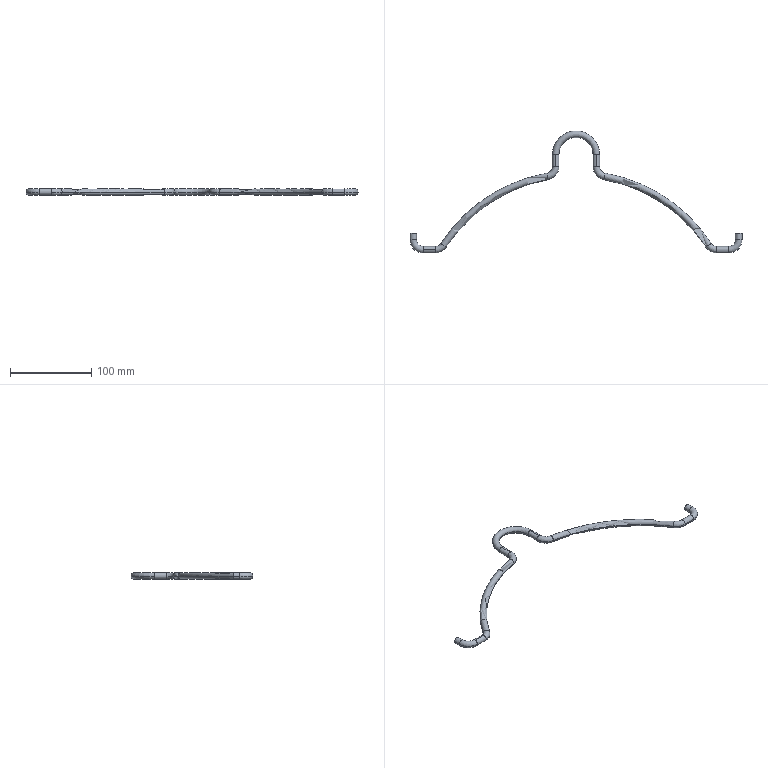Part | STEP file | HXGR200008-05-20-03 | 1 solid | 32 faces | box 408 x 150 x 8 mm | volume 28410 mm3 | torus 18 | cylinder 12 | plane 2 | commonest cylinder face diameters 8 x12
STEP:
#1=CARTESIAN_POINT('',(-196.,113.666,0.));
#2=VERTEX_POINT('',#1);
#3=CARTESIAN_POINT('',(-204.,113.666,0.));
#4=VERTEX_POINT('',#3);
#5=CARTESIAN_POINT('',(-200.,113.666,0.));
#6=DIRECTION('',(0.,-1.,0.));
#7=DIRECTION('',(1.,0.,0.));
#8=AXIS2_PLACEMENT_3D('',#5,#6,#7);
#9=CIRCLE('',#8,4.);
#10=EDGE_CURVE('',#2,#4,#9,.T.);
#11=ORIENTED_EDGE('',*,*,#10,.T.);
#12=CARTESIAN_POINT('',(-188.,97.666,0.));
#13=VERTEX_POINT('',#12);
#14=CARTESIAN_POINT('',(-188.,113.666,0.));
#15=DIRECTION('',(0.,0.,1.));
#16=DIRECTION('',(0.,-1.,0.));
#17=AXIS2_PLACEMENT_3D('',#14,#15,#16);
#18=CIRCLE('',#17,16.);
#19=EDGE_CURVE('',#4,#13,#18,.T.);
#20=ORIENTED_EDGE('',*,*,#19,.T.);
#21=CARTESIAN_POINT('',(-188.,101.666,4.));
#22=VERTEX_POINT('',#21);
#23=CARTESIAN_POINT('',(-188.,101.666,0.));
#24=DIRECTION('',(1.,0.,0.));
#25=DIRECTION('',(0.,1.,0.));
#26=AXIS2_PLACEMENT_3D('',#23,#24,#25);
#27=CIRCLE('',#26,4.);
#28=EDGE_CURVE('',#22,#13,#27,.T.);
#29=ORIENTED_EDGE('',*,*,#28,.F.);
#30=CARTESIAN_POINT('',(-188.,105.666,0.));
#31=VERTEX_POINT('',#30);
#32=CARTESIAN_POINT('',(-188.,101.666,0.));
#33=DIRECTION('',(1.,0.,0.));
#34=DIRECTION('',(0.,1.,0.));
#35=AXIS2_PLACEMENT_3D('',#32,#33,#34);
#36=CIRCLE('',#35,4.);
#37=EDGE_CURVE('',#31,#22,#36,.T.);
#38=ORIENTED_EDGE('',*,*,#37,.F.);
#39=CARTESIAN_POINT('',(-188.,113.666,0.));
#40=DIRECTION('',(0.,0.,1.));
#41=DIRECTION('',(0.,-1.,0.));
#42=AXIS2_PLACEMENT_3D('',#39,#40,#41);
#43=CIRCLE('',#42,8.);
#44=EDGE_CURVE('',#2,#31,#43,.T.);
#45=ORIENTED_EDGE('',*,*,#44,.F.);
#46=EDGE_LOOP('',(#11,#20,#29,#38,#45));
#47=FACE_OUTER_BOUND('',#46,.T.);
#48=CARTESIAN_POINT('',(-188.,113.666,0.));
#49=DIRECTION('',(0.,0.,1.));
#50=DIRECTION('',(1.,0.,0.));
#51=AXIS2_PLACEMENT_3D('',#48,#49,#50);
#52=TOROIDAL_SURFACE('',#51,12.,4.);
#53=ADVANCED_FACE('',(#47),#52,.T.);
#54=CARTESIAN_POINT('',(-173.,101.666,4.));
#55=VERTEX_POINT('',#54);
#56=CARTESIAN_POINT('',(-173.,97.666,0.));
#57=VERTEX_POINT('',#56);
#58=CARTESIAN_POINT('',(-173.,101.666,0.));
#59=DIRECTION('',(1.,0.,0.));
#60=DIRECTION('',(0.,1.,0.));
#61=AXIS2_PLACEMENT_3D('',#58,#59,#60);
#62=CIRCLE('',#61,4.);
#63=EDGE_CURVE('',#55,#57,#62,.T.);
#64=ORIENTED_EDGE('',*,*,#63,.T.);
#65=CARTESIAN_POINT('',(-159.628,104.88,0.));
#66=VERTEX_POINT('',#65);
#67=CARTESIAN_POINT('',(-173.,113.666,0.));
#68=DIRECTION('',(0.,0.,1.));
#69=DIRECTION('',(0.,-1.,0.));
#70=AXIS2_PLACEMENT_3D('',#67,#68,#69);
#71=CIRCLE('',#70,16.);
#72=EDGE_CURVE('',#57,#66,#71,.T.);
#73=ORIENTED_EDGE('',*,*,#72,.T.);
#74=CARTESIAN_POINT('',(-166.314,109.273,0.));
#75=VERTEX_POINT('',#74);
#76=CARTESIAN_POINT('',(-162.971,107.077,0.));
#77=DIRECTION('',(0.5491,0.8357,0.));
#78=DIRECTION('',(-0.8357,0.5491,0.));
#79=AXIS2_PLACEMENT_3D('',#76,#77,#78);
#80=CIRCLE('',#79,4.);
#81=EDGE_CURVE('',#75,#66,#80,.T.);
#82=ORIENTED_EDGE('',*,*,#81,.F.);
#83=CARTESIAN_POINT('',(-173.,105.666,0.));
#84=VERTEX_POINT('',#83);
#85=CARTESIAN_POINT('',(-173.,113.666,0.));
#86=DIRECTION('',(0.,0.,1.));
#87=DIRECTION('',(0.,-1.,0.));
#88=AXIS2_PLACEMENT_3D('',#85,#86,#87);
#89=CIRCLE('',#88,8.);
#90=EDGE_CURVE('',#84,#75,#89,.T.);
#91=ORIENTED_EDGE('',*,*,#90,.F.);
#92=CARTESIAN_POINT('',(-173.,101.666,0.));
#93=DIRECTION('',(1.,0.,0.));
#94=DIRECTION('',(0.,1.,0.));
#95=AXIS2_PLACEMENT_3D('',#92,#93,#94);
#96=CIRCLE('',#95,4.);
#97=EDGE_CURVE('',#84,#55,#96,.T.);
#98=ORIENTED_EDGE('',*,*,#97,.T.);
#99=EDGE_LOOP('',(#64,#73,#82,#91,#98));
#100=FACE_OUTER_BOUND('',#99,.T.);
#101=CARTESIAN_POINT('',(-173.,113.666,0.));
#102=DIRECTION('',(0.,0.,1.));
#103=DIRECTION('',(1.,0.,0.));
#104=AXIS2_PLACEMENT_3D('',#101,#102,#103);
#105=TOROIDAL_SURFACE('',#104,12.,4.);
#106=ADVANCED_FACE('',(#100),#105,.T.);
#107=CARTESIAN_POINT('',(-162.971,107.077,0.));
#108=DIRECTION('',(0.5491,0.8357,0.));
#109=DIRECTION('',(-0.8357,0.5491,0.));
#110=AXIS2_PLACEMENT_3D('',#107,#108,#109);
#111=CIRCLE('',#110,4.);
#112=EDGE_CURVE('',#66,#75,#111,.T.);
#113=ORIENTED_EDGE('',*,*,#112,.T.);
#114=CARTESIAN_POINT('',(-35.57,195.795,0.));
#115=VERTEX_POINT('',#114);
#116=CARTESIAN_POINT('',(0.,0.,0.));
#117=DIRECTION('',(0.,0.,-1.));
#118=DIRECTION('',(0.,1.,0.));
#119=AXIS2_PLACEMENT_3D('',#116,#117,#118);
#120=CIRCLE('',#119,199.);
#121=EDGE_CURVE('',#75,#115,#120,.T.);
#122=ORIENTED_EDGE('',*,*,#121,.T.);
#123=CARTESIAN_POINT('',(-34.14,187.924,0.));
#124=VERTEX_POINT('',#123);
#125=CARTESIAN_POINT('',(-34.855,191.86,0.));
#126=DIRECTION('',(0.9839,0.1787,0.));
#127=DIRECTION('',(-0.1787,0.9839,0.));
#128=AXIS2_PLACEMENT_3D('',#125,#126,#127);
#129=CIRCLE('',#128,4.);
#130=EDGE_CURVE('',#124,#115,#129,.T.);
#131=ORIENTED_EDGE('',*,*,#130,.F.);
#132=CARTESIAN_POINT('',(0.,0.,0.));
#133=DIRECTION('',(0.,0.,-1.));
#134=DIRECTION('',(0.,1.,0.));
#135=AXIS2_PLACEMENT_3D('',#132,#133,#134);
#136=CIRCLE('',#135,191.);
#137=EDGE_CURVE('',#66,#124,#136,.T.);
#138=ORIENTED_EDGE('',*,*,#137,.F.);
#139=EDGE_LOOP('',(#113,#122,#131,#138));
#140=FACE_OUTER_BOUND('',#139,.T.);
#141=CARTESIAN_POINT('',(0.,0.,0.));
#142=DIRECTION('',(0.,0.,-1.));
#143=DIRECTION('',(-1.,0.,0.));
#144=AXIS2_PLACEMENT_3D('',#141,#142,#143);
#145=TOROIDAL_SURFACE('',#144,195.,4.);
#146=ADVANCED_FACE('',(#140),#145,.T.);
#147=CARTESIAN_POINT('',(-34.855,191.86,0.));
#148=DIRECTION('',(0.9839,0.1787,0.));
#149=DIRECTION('',(-0.1787,0.9839,0.));
#150=AXIS2_PLACEMENT_3D('',#147,#148,#149);
#151=CIRCLE('',#150,4.);
#152=EDGE_CURVE('',#115,#124,#151,.T.);
#153=ORIENTED_EDGE('',*,*,#152,.T.);
#154=CARTESIAN_POINT('',(-21.,203.666,0.));
#155=VERTEX_POINT('',#154);
#156=CARTESIAN_POINT('',(-37.,203.666,0.));
#157=DIRECTION('',(0.,0.,1.));
#158=DIRECTION('',(0.,-1.,0.));
#159=AXIS2_PLACEMENT_3D('',#156,#157,#158);
#160=CIRCLE('',#159,16.);
#161=EDGE_CURVE('',#124,#155,#160,.T.);
#162=ORIENTED_EDGE('',*,*,#161,.T.);
#163=CARTESIAN_POINT('',(-25.,203.666,4.));
#164=VERTEX_POINT('',#163);
#165=CARTESIAN_POINT('',(-25.,203.666,0.));
#166=DIRECTION('',(0.,1.,0.));
#167=DIRECTION('',(-1.,0.,0.));
#168=AXIS2_PLACEMENT_3D('',#165,#166,#167);
#169=CIRCLE('',#168,4.);
#170=EDGE_CURVE('',#164,#155,#169,.T.);
#171=ORIENTED_EDGE('',*,*,#170,.F.);
#172=CARTESIAN_POINT('',(-29.,203.666,0.));
#173=VERTEX_POINT('',#172);
#174=CARTESIAN_POINT('',(-25.,203.666,0.));
#175=DIRECTION('',(0.,1.,0.));
#176=DIRECTION('',(-1.,0.,0.));
#177=AXIS2_PLACEMENT_3D('',#174,#175,#176);
#178=CIRCLE('',#177,4.);
#179=EDGE_CURVE('',#173,#164,#178,.T.);
#180=ORIENTED_EDGE('',*,*,#179,.F.);
#181=CARTESIAN_POINT('',(-37.,203.666,0.));
#182=DIRECTION('',(0.,0.,1.));
#183=DIRECTION('',(0.,-1.,0.));
#184=AXIS2_PLACEMENT_3D('',#181,#182,#183);
#185=CIRCLE('',#184,8.);
#186=EDGE_CURVE('',#115,#173,#185,.T.);
#187=ORIENTED_EDGE('',*,*,#186,.F.);
#188=EDGE_LOOP('',(#153,#162,#171,#180,#187));
#189=FACE_OUTER_BOUND('',#188,.T.);
#190=CARTESIAN_POINT('',(-37.,203.666,0.));
#191=DIRECTION('',(0.,0.,1.));
#192=DIRECTION('',(1.,0.,0.));
#193=AXIS2_PLACEMENT_3D('',#190,#191,#192);
#194=TOROIDAL_SURFACE('',#193,12.,4.);
#195=ADVANCED_FACE('',(#189),#194,.T.);
#196=CARTESIAN_POINT('',(-25.,218.666,-4.));
#197=VERTEX_POINT('',#196);
#198=CARTESIAN_POINT('',(-29.,218.666,0.));
#199=VERTEX_POINT('',#198);
#200=CARTESIAN_POINT('',(-25.,218.666,0.));
#201=DIRECTION('',(0.,1.,0.));
#202=DIRECTION('',(-1.,0.,0.));
#203=AXIS2_PLACEMENT_3D('',#200,#201,#202);
#204=CIRCLE('',#203,4.);
#205=EDGE_CURVE('',#197,#199,#204,.T.);
#206=ORIENTED_EDGE('',*,*,#205,.T.);
#207=CARTESIAN_POINT('',(29.,218.666,0.));
#208=VERTEX_POINT('',#207);
#209=CARTESIAN_POINT('',(0.,218.666,0.));
#210=DIRECTION('',(0.,0.,-1.));
#211=DIRECTION('',(0.,1.,0.));
#212=AXIS2_PLACEMENT_3D('',#209,#210,#211);
#213=CIRCLE('',#212,29.);
#214=EDGE_CURVE('',#199,#208,#213,.T.);
#215=ORIENTED_EDGE('',*,*,#214,.T.);
#216=CARTESIAN_POINT('',(25.,218.666,-4.));
#217=VERTEX_POINT('',#216);
#218=CARTESIAN_POINT('',(25.,218.666,0.));
#219=DIRECTION('',(0.,-1.,0.));
#220=DIRECTION('',(1.,0.,0.));
#221=AXIS2_PLACEMENT_3D('',#218,#219,#220);
#222=CIRCLE('',#221,4.);
#223=EDGE_CURVE('',#217,#208,#222,.T.);
#224=ORIENTED_EDGE('',*,*,#223,.F.);
#225=CARTESIAN_POINT('',(21.,218.666,0.));
#226=VERTEX_POINT('',#225);
#227=CARTESIAN_POINT('',(25.,218.666,0.));
#228=DIRECTION('',(0.,-1.,0.));
#229=DIRECTION('',(1.,0.,0.));
#230=AXIS2_PLACEMENT_3D('',#227,#228,#229);
#231=CIRCLE('',#230,4.);
#232=EDGE_CURVE('',#226,#217,#231,.T.);
#233=ORIENTED_EDGE('',*,*,#232,.F.);
#234=CARTESIAN_POINT('',(-21.,218.666,0.));
#235=VERTEX_POINT('',#234);
#236=CARTESIAN_POINT('',(0.,218.666,0.));
#237=DIRECTION('',(0.,0.,-1.));
#238=DIRECTION('',(0.,1.,0.));
#239=AXIS2_PLACEMENT_3D('',#236,#237,#238);
#240=CIRCLE('',#239,21.);
#241=EDGE_CURVE('',#235,#226,#240,.T.);
#242=ORIENTED_EDGE('',*,*,#241,.F.);
#243=CARTESIAN_POINT('',(-25.,218.666,0.));
#244=DIRECTION('',(0.,1.,0.));
#245=DIRECTION('',(-1.,0.,0.));
#246=AXIS2_PLACEMENT_3D('',#243,#244,#245);
#247=CIRCLE('',#246,4.);
#248=EDGE_CURVE('',#235,#197,#247,.T.);
#249=ORIENTED_EDGE('',*,*,#248,.T.);
#250=EDGE_LOOP('',(#206,#215,#224,#233,#242,#249));
#251=FACE_OUTER_BOUND('',#250,.T.);
#252=CARTESIAN_POINT('',(0.,218.666,0.));
#253=DIRECTION('',(0.,0.,-1.));
#254=DIRECTION('',(-1.,0.,0.));
#255=AXIS2_PLACEMENT_3D('',#252,#253,#254);
#256=TOROIDAL_SURFACE('',#255,25.,4.);
#257=ADVANCED_FACE('',(#251),#256,.T.);
#258=CARTESIAN_POINT('',(25.,203.666,4.));
#259=VERTEX_POINT('',#258);
#260=CARTESIAN_POINT('',(21.,203.666,0.));
#261=VERTEX_POINT('',#260);
#262=CARTESIAN_POINT('',(25.,203.666,0.));
#263=DIRECTION('',(0.,-1.,0.));
#264=DIRECTION('',(1.,0.,0.));
#265=AXIS2_PLACEMENT_3D('',#262,#263,#264);
#266=CIRCLE('',#265,4.);
#267=EDGE_CURVE('',#259,#261,#266,.T.);
#268=ORIENTED_EDGE('',*,*,#267,.T.);
#269=CARTESIAN_POINT('',(34.14,187.924,0.));
#270=VERTEX_POINT('',#269);
#271=CARTESIAN_POINT('',(37.,203.666,0.));
#272=DIRECTION('',(0.,0.,1.));
#273=DIRECTION('',(0.,-1.,0.));
#274=AXIS2_PLACEMENT_3D('',#271,#272,#273);
#275=CIRCLE('',#274,16.);
#276=EDGE_CURVE('',#261,#270,#275,.T.);
#277=ORIENTED_EDGE('',*,*,#276,.T.);
#278=CARTESIAN_POINT('',(35.57,195.795,0.));
#279=VERTEX_POINT('',#278);
#280=CARTESIAN_POINT('',(34.855,191.86,0.));
#281=DIRECTION('',(0.9839,-0.1787,0.));
#282=DIRECTION('',(0.1787,0.9839,0.));
#283=AXIS2_PLACEMENT_3D('',#280,#281,#282);
#284=CIRCLE('',#283,4.);
#285=EDGE_CURVE('',#279,#270,#284,.T.);
#286=ORIENTED_EDGE('',*,*,#285,.F.);
#287=CARTESIAN_POINT('',(29.,203.666,0.));
#288=VERTEX_POINT('',#287);
#289=CARTESIAN_POINT('',(37.,203.666,0.));
#290=DIRECTION('',(0.,0.,1.));
#291=DIRECTION('',(0.,-1.,0.));
#292=AXIS2_PLACEMENT_3D('',#289,#290,#291);
#293=CIRCLE('',#292,8.);
#294=EDGE_CURVE('',#288,#279,#293,.T.);
#295=ORIENTED_EDGE('',*,*,#294,.F.);
#296=CARTESIAN_POINT('',(25.,203.666,0.));
#297=DIRECTION('',(0.,-1.,0.));
#298=DIRECTION('',(1.,0.,0.));
#299=AXIS2_PLACEMENT_3D('',#296,#297,#298);
#300=CIRCLE('',#299,4.);
#301=EDGE_CURVE('',#288,#259,#300,.T.);
#302=ORIENTED_EDGE('',*,*,#301,.T.);
#303=EDGE_LOOP('',(#268,#277,#286,#295,#302));
#304=FACE_OUTER_BOUND('',#303,.T.);
#305=CARTESIAN_POINT('',(37.,203.666,0.));
#306=DIRECTION('',(0.,0.,1.));
#307=DIRECTION('',(1.,0.,0.));
#308=AXIS2_PLACEMENT_3D('',#305,#306,#307);
#309=TOROIDAL_SURFACE('',#308,12.,4.);
#310=ADVANCED_FACE('',(#304),#309,.T.);
#311=CARTESIAN_POINT('',(34.855,191.86,0.));
#312=DIRECTION('',(0.9839,-0.1787,0.));
#313=DIRECTION('',(0.1787,0.9839,0.));
#314=AXIS2_PLACEMENT_3D('',#311,#312,#313);
#315=CIRCLE('',#314,4.);
#316=EDGE_CURVE('',#270,#279,#315,.T.);
#317=ORIENTED_EDGE('',*,*,#316,.T.);
#318=CARTESIAN_POINT('',(166.314,109.273,0.));
#319=VERTEX_POINT('',#318);
#320=CARTESIAN_POINT('',(0.,0.,0.));
#321=DIRECTION('',(0.,0.,-1.));
#322=DIRECTION('',(0.,1.,0.));
#323=AXIS2_PLACEMENT_3D('',#320,#321,#322);
#324=CIRCLE('',#323,199.);
#325=EDGE_CURVE('',#279,#319,#324,.T.);
#326=ORIENTED_EDGE('',*,*,#325,.T.);
#327=CARTESIAN_POINT('',(159.628,104.88,0.));
#328=VERTEX_POINT('',#327);
#329=CARTESIAN_POINT('',(162.971,107.077,0.));
#330=DIRECTION('',(0.5491,-0.8357,0.));
#331=DIRECTION('',(0.8357,0.5491,0.));
#332=AXIS2_PLACEMENT_3D('',#329,#330,#331);
#333=CIRCLE('',#332,4.);
#334=EDGE_CURVE('',#328,#319,#333,.T.);
#335=ORIENTED_EDGE('',*,*,#334,.F.);
#336=CARTESIAN_POINT('',(0.,0.,0.));
#337=DIRECTION('',(0.,0.,-1.));
#338=DIRECTION('',(0.,1.,0.));
#339=AXIS2_PLACEMENT_3D('',#336,#337,#338);
#340=CIRCLE('',#339,191.);
#341=EDGE_CURVE('',#270,#328,#340,.T.);
#342=ORIENTED_EDGE('',*,*,#341,.F.);
#343=EDGE_LOOP('',(#317,#326,#335,#342));
#344=FACE_OUTER_BOUND('',#343,.T.);
#345=CARTESIAN_POINT('',(0.,0.,0.));
#346=DIRECTION('',(0.,0.,-1.));
#347=DIRECTION('',(-1.,0.,0.));
#348=AXIS2_PLACEMENT_3D('',#345,#346,#347);
#349=TOROIDAL_SURFACE('',#348,195.,4.);
#350=ADVANCED_FACE('',(#344),#349,.T.);
#351=CARTESIAN_POINT('',(162.971,107.077,0.));
#352=DIRECTION('',(0.5491,-0.8357,0.));
#353=DIRECTION('',(0.8357,0.5491,0.));
#354=AXIS2_PLACEMENT_3D('',#351,#352,#353);
#355=CIRCLE('',#354,4.);
#356=EDGE_CURVE('',#319,#328,#355,.T.);
#357=ORIENTED_EDGE('',*,*,#356,.T.);
#358=CARTESIAN_POINT('',(173.,97.666,0.));
#359=VERTEX_POINT('',#358);
#360=CARTESIAN_POINT('',(173.,113.666,0.));
#361=DIRECTION('',(0.,0.,1.));
#362=DIRECTION('',(0.,-1.,0.));
#363=AXIS2_PLACEMENT_3D('',#360,#361,#362);
#364=CIRCLE('',#363,16.);
#365=EDGE_CURVE('',#328,#359,#364,.T.);
#366=ORIENTED_EDGE('',*,*,#365,.T.);
#367=CARTESIAN_POINT('',(173.,105.666,0.));
#368=VERTEX_POINT('',#367);
#369=CARTESIAN_POINT('',(173.,101.666,0.));
#370=DIRECTION('',(1.,0.,0.));
#371=DIRECTION('',(0.,1.,0.));
#372=AXIS2_PLACEMENT_3D('',#369,#370,#371);
#373=CIRCLE('',#372,4.);
#374=EDGE_CURVE('',#368,#359,#373,.T.);
#375=ORIENTED_EDGE('',*,*,#374,.F.);
#376=CARTESIAN_POINT('',(173.,113.666,0.));
#377=DIRECTION('',(0.,0.,1.));
#378=DIRECTION('',(0.,-1.,0.));
#379=AXIS2_PLACEMENT_3D('',#376,#377,#378);
#380=CIRCLE('',#379,8.);
#381=EDGE_CURVE('',#319,#368,#380,.T.);
#382=ORIENTED_EDGE('',*,*,#381,.F.);
#383=EDGE_LOOP('',(#357,#366,#375,#382));
#384=FACE_OUTER_BOUND('',#383,.T.);
#385=CARTESIAN_POINT('',(173.,113.666,0.));
#386=DIRECTION('',(0.,0.,1.));
#387=DIRECTION('',(1.,0.,0.));
#388=AXIS2_PLACEMENT_3D('',#385,#386,#387);
#389=TOROIDAL_SURFACE('',#388,12.,4.);
#390=ADVANCED_FACE('',(#384),#389,.T.);
#391=CARTESIAN_POINT('',(188.,105.666,0.));
#392=VERTEX_POINT('',#391);
#393=CARTESIAN_POINT('',(188.,97.666,0.));
#394=VERTEX_POINT('',#393);
#395=CARTESIAN_POINT('',(188.,101.666,0.));
#396=DIRECTION('',(1.,0.,0.));
#397=DIRECTION('',(0.,1.,0.));
#398=AXIS2_PLACEMENT_3D('',#395,#396,#397);
#399=CIRCLE('',#398,4.);
#400=EDGE_CURVE('',#392,#394,#399,.T.);
#401=ORIENTED_EDGE('',*,*,#400,.T.);
#402=CARTESIAN_POINT('',(204.,113.666,0.));
#403=VERTEX_POINT('',#402);
#404=CARTESIAN_POINT('',(188.,113.666,0.));
#405=DIRECTION('',(0.,0.,1.));
#406=DIRECTION('',(0.,-1.,0.));
#407=AXIS2_PLACEMENT_3D('',#404,#405,#406);
#408=CIRCLE('',#407,16.);
#409=EDGE_CURVE('',#394,#403,#408,.T.);
#410=ORIENTED_EDGE('',*,*,#409,.T.);
#411=CARTESIAN_POINT('',(196.,113.666,0.));
#412=VERTEX_POINT('',#411);
#413=CARTESIAN_POINT('',(200.,113.666,0.));
#414=DIRECTION('',(0.,1.,0.));
#415=DIRECTION('',(-1.,0.,0.));
#416=AXIS2_PLACEMENT_3D('',#413,#414,#415);
#417=CIRCLE('',#416,4.);
#418=EDGE_CURVE('',#412,#403,#417,.T.);
#419=ORIENTED_EDGE('',*,*,#418,.F.);
#420=CARTESIAN_POINT('',(188.,113.666,0.));
#421=DIRECTION('',(0.,0.,1.));
#422=DIRECTION('',(0.,-1.,0.));
#423=AXIS2_PLACEMENT_3D('',#420,#421,#422);
#424=CIRCLE('',#423,8.);
#425=EDGE_CURVE('',#392,#412,#424,.T.);
#426=ORIENTED_EDGE('',*,*,#425,.F.);
#427=EDGE_LOOP('',(#401,#410,#419,#426));
#428=FACE_OUTER_BOUND('',#427,.T.);
#429=CARTESIAN_POINT('',(188.,113.666,0.));
#430=DIRECTION('',(0.,0.,1.));
#431=DIRECTION('',(1.,0.,0.));
#432=AXIS2_PLACEMENT_3D('',#429,#430,#431);
#433=TOROIDAL_SURFACE('',#432,12.,4.);
#434=ADVANCED_FACE('',(#428),#433,.T.);
#435=ORIENTED_EDGE('',*,*,#10,.F.);
#436=CARTESIAN_POINT('',(-196.,121.666,0.));
#437=VERTEX_POINT('',#436);
#438=CARTESIAN_POINT('',(-196.,113.666,0.));
#439=DIRECTION('',(0.,1.,0.));
#440=VECTOR('',#439,1000.);
#441=LINE('',#438,#440);
#442=EDGE_CURVE('',#2,#437,#441,.T.);
#443=ORIENTED_EDGE('',*,*,#442,.T.);
#444=CARTESIAN_POINT('',(-204.,121.666,0.));
#445=VERTEX_POINT('',#444);
#446=CARTESIAN_POINT('',(-200.,121.666,0.));
#447=DIRECTION('',(0.,-1.,0.));
#448=DIRECTION('',(1.,0.,0.));
#449=AXIS2_PLACEMENT_3D('',#446,#447,#448);
#450=CIRCLE('',#449,4.);
#451=EDGE_CURVE('',#437,#445,#450,.T.);
#452=ORIENTED_EDGE('',*,*,#451,.T.);
#453=CARTESIAN_POINT('',(-204.,113.666,0.));
#454=DIRECTION('',(0.,1.,0.));
#455=VECTOR('',#454,1000.);
#456=LINE('',#453,#455);
#457=EDGE_CURVE('',#4,#445,#456,.T.);
#458=ORIENTED_EDGE('',*,*,#457,.F.);
#459=EDGE_LOOP('',(#435,#443,#452,#458));
#460=FACE_OUTER_BOUND('',#459,.T.);
#461=CARTESIAN_POINT('',(-200.,113.666,0.));
#462=DIRECTION('',(0.,1.,0.));
#463=DIRECTION('',(-1.,0.,0.));
#464=AXIS2_PLACEMENT_3D('',#461,#462,#463);
#465=CYLINDRICAL_SURFACE('',#464,4.);
#466=ADVANCED_FACE('',(#460),#465,.T.);
#467=CARTESIAN_POINT('',(-188.,101.666,-4.));
#468=VERTEX_POINT('',#467);
#469=CARTESIAN_POINT('',(-188.,101.666,0.));
#470=DIRECTION('',(1.,0.,0.));
#471=DIRECTION('',(0.,1.,0.));
#472=AXIS2_PLACEMENT_3D('',#469,#470,#471);
#473=CIRCLE('',#472,4.);
#474=EDGE_CURVE('',#468,#31,#473,.T.);
#475=ORIENTED_EDGE('',*,*,#474,.T.);
#476=ORIENTED_EDGE('',*,*,#37,.T.);
#477=CARTESIAN_POINT('',(-188.,101.666,4.));
#478=DIRECTION('',(1.,0.,0.));
#479=VECTOR('',#478,1000.);
#480=LINE('',#477,#479);
#481=EDGE_CURVE('',#22,#55,#480,.T.);
#482=ORIENTED_EDGE('',*,*,#481,.T.);
#483=ORIENTED_EDGE('',*,*,#97,.F.);
#484=CARTESIAN_POINT('',(-173.,101.666,-4.));
#485=VERTEX_POINT('',#484);
#486=CARTESIAN_POINT('',(-173.,101.666,0.));
#487=DIRECTION('',(1.,0.,0.));
#488=DIRECTION('',(0.,1.,0.));
#489=AXIS2_PLACEMENT_3D('',#486,#487,#488);
#490=CIRCLE('',#489,4.);
#491=EDGE_CURVE('',#485,#84,#490,.T.);
#492=ORIENTED_EDGE('',*,*,#491,.F.);
#493=CARTESIAN_POINT('',(-188.,101.666,-4.));
#494=DIRECTION('',(1.,0.,0.));
#495=VECTOR('',#494,1000.);
#496=LINE('',#493,#495);
#497=EDGE_CURVE('',#468,#485,#496,.T.);
#498=ORIENTED_EDGE('',*,*,#497,.F.);
#499=EDGE_LOOP('',(#475,#476,#482,#483,#492,#498));
#500=FACE_OUTER_BOUND('',#499,.T.);
#501=CARTESIAN_POINT('',(-188.,101.666,0.));
#502=DIRECTION('',(1.,0.,0.));
#503=DIRECTION('',(0.,0.,-1.));
#504=AXIS2_PLACEMENT_3D('',#501,#502,#503);
#505=CYLINDRICAL_SURFACE('',#504,4.);
#506=ADVANCED_FACE('',(#500),#505,.T.);
#507=ORIENTED_EDGE('',*,*,#170,.T.);
#508=CARTESIAN_POINT('',(-25.,203.666,-4.));
#509=VERTEX_POINT('',#508);
#510=CARTESIAN_POINT('',(-25.,203.666,0.));
#511=DIRECTION('',(0.,1.,0.));
#512=DIRECTION('',(-1.,0.,0.));
#513=AXIS2_PLACEMENT_3D('',#510,#511,#512);
#514=CIRCLE('',#513,4.);
#515=EDGE_CURVE('',#155,#509,#514,.T.);
#516=ORIENTED_EDGE('',*,*,#515,.T.);
#517=CARTESIAN_POINT('',(-25.,203.666,-4.));
#518=DIRECTION('',(0.,1.,0.));
#519=VECTOR('',#518,1000.);
#520=LINE('',#517,#519);
#521=EDGE_CURVE('',#509,#197,#520,.T.);
#522=ORIENTED_EDGE('',*,*,#521,.T.);
#523=ORIENTED_EDGE('',*,*,#248,.F.);
#524=CARTESIAN_POINT('',(-25.,218.666,4.));
#525=VERTEX_POINT('',#524);
#526=CARTESIAN_POINT('',(-25.,218.666,0.));
#527=DIRECTION('',(0.,1.,0.));
#528=DIRECTION('',(-1.,0.,0.));
#529=AXIS2_PLACEMENT_3D('',#526,#527,#528);
#530=CIRCLE('',#529,4.);
#531=EDGE_CURVE('',#525,#235,#530,.T.);
#532=ORIENTED_EDGE('',*,*,#531,.F.);
#533=CARTESIAN_POINT('',(-25.,203.666,4.));
#534=DIRECTION('',(0.,1.,0.));
#535=VECTOR('',#534,1000.);
#536=LINE('',#533,#535);
#537=EDGE_CURVE('',#164,#525,#536,.T.);
#538=ORIENTED_EDGE('',*,*,#537,.F.);
#539=EDGE_LOOP('',(#507,#516,#522,#523,#532,#538));
#540=FACE_OUTER_BOUND('',#539,.T.);
#541=CARTESIAN_POINT('',(-25.,203.666,0.));
#542=DIRECTION('',(0.,1.,0.));
#543=DIRECTION('',(0.,0.,1.));
#544=AXIS2_PLACEMENT_3D('',#541,#542,#543);
#545=CYLINDRICAL_SURFACE('',#544,4.);
#546=ADVANCED_FACE('',(#540),#545,.T.);
#547=ORIENTED_EDGE('',*,*,#223,.T.);
#548=CARTESIAN_POINT('',(25.,218.666,4.));
#549=VERTEX_POINT('',#548);
#550=CARTESIAN_POINT('',(25.,218.666,0.));
#551=DIRECTION('',(0.,-1.,0.));
#552=DIRECTION('',(1.,0.,0.));
#553=AXIS2_PLACEMENT_3D('',#550,#551,#552);
#554=CIRCLE('',#553,4.);
#555=EDGE_CURVE('',#208,#549,#554,.T.);
#556=ORIENTED_EDGE('',*,*,#555,.T.);
#557=CARTESIAN_POINT('',(25.,218.666,4.));
#558=DIRECTION('',(0.,-1.,0.));
#559=VECTOR('',#558,1000.);
#560=LINE('',#557,#559);
#561=EDGE_CURVE('',#549,#259,#560,.T.);
#562=ORIENTED_EDGE('',*,*,#561,.T.);
#563=ORIENTED_EDGE('',*,*,#301,.F.);
#564=CARTESIAN_POINT('',(25.,203.666,-4.));
#565=VERTEX_POINT('',#564);
#566=CARTESIAN_POINT('',(25.,203.666,0.));
#567=DIRECTION('',(0.,-1.,0.));
#568=DIRECTION('',(1.,0.,0.));
#569=AXIS2_PLACEMENT_3D('',#566,#567,#568);
#570=CIRCLE('',#569,4.);
#571=EDGE_CURVE('',#565,#288,#570,.T.);
#572=ORIENTED_EDGE('',*,*,#571,.F.);
#573=CARTESIAN_POINT('',(25.,218.666,-4.));
#574=DIRECTION('',(0.,-1.,0.));
#575=VECTOR('',#574,1000.);
#576=LINE('',#573,#575);
#577=EDGE_CURVE('',#217,#565,#576,.T.);
#578=ORIENTED_EDGE('',*,*,#577,.F.);
#579=EDGE_LOOP('',(#547,#556,#562,#563,#572,#578));
#580=FACE_OUTER_BOUND('',#579,.T.);
#581=CARTESIAN_POINT('',(25.,218.666,0.));
#582=DIRECTION('',(0.,-1.,0.));
#583=DIRECTION('',(0.,0.,-1.));
#584=AXIS2_PLACEMENT_3D('',#581,#582,#583);
#585=CYLINDRICAL_SURFACE('',#584,4.);
#586=ADVANCED_FACE('',(#580),#585,.T.);
#587=ORIENTED_EDGE('',*,*,#374,.T.);
#588=CARTESIAN_POINT('',(173.,97.666,0.));
#589=DIRECTION('',(1.,0.,0.));
#590=VECTOR('',#589,1000.);
#591=LINE('',#588,#590);
#592=EDGE_CURVE('',#359,#394,#591,.T.);
#593=ORIENTED_EDGE('',*,*,#592,.T.);
#594=ORIENTED_EDGE('',*,*,#400,.F.);
#595=CARTESIAN_POINT('',(173.,105.666,0.));
#596=DIRECTION('',(1.,0.,0.));
#597=VECTOR('',#596,1000.);
#598=LINE('',#595,#597);
#599=EDGE_CURVE('',#368,#392,#598,.T.);
#600=ORIENTED_EDGE('',*,*,#599,.F.);
#601=EDGE_LOOP('',(#587,#593,#594,#600));
#602=FACE_OUTER_BOUND('',#601,.T.);
#603=CARTESIAN_POINT('',(173.,101.666,0.));
#604=DIRECTION('',(1.,0.,0.));
#605=DIRECTION('',(0.,1.,0.));
#606=AXIS2_PLACEMENT_3D('',#603,#604,#605);
#607=CYLINDRICAL_SURFACE('',#606,4.);
#608=ADVANCED_FACE('',(#602),#607,.T.);
#609=ORIENTED_EDGE('',*,*,#418,.T.);
#610=CARTESIAN_POINT('',(204.,121.666,0.));
#611=VERTEX_POINT('',#610);
#612=CARTESIAN_POINT('',(204.,113.666,0.));
#613=DIRECTION('',(0.,1.,0.));
#614=VECTOR('',#613,1000.);
#615=LINE('',#612,#614);
#616=EDGE_CURVE('',#403,#611,#615,.T.);
#617=ORIENTED_EDGE('',*,*,#616,.T.);
#618=CARTESIAN_POINT('',(196.,121.666,0.));
#619=VERTEX_POINT('',#618);
#620=CARTESIAN_POINT('',(200.,121.666,0.));
#621=DIRECTION('',(0.,1.,0.));
#622=DIRECTION('',(-1.,0.,0.));
#623=AXIS2_PLACEMENT_3D('',#620,#621,#622);
#624=CIRCLE('',#623,4.);
#625=EDGE_CURVE('',#619,#611,#624,.T.);
#626=ORIENTED_EDGE('',*,*,#625,.F.);
#627=CARTESIAN_POINT('',(196.,113.666,0.));
#628=DIRECTION('',(0.,1.,0.));
#629=VECTOR('',#628,1000.);
#630=LINE('',#627,#629);
#631=EDGE_CURVE('',#412,#619,#630,.T.);
#632=ORIENTED_EDGE('',*,*,#631,.F.);
#633=EDGE_LOOP('',(#609,#617,#626,#632));
#634=FACE_OUTER_BOUND('',#633,.T.);
#635=CARTESIAN_POINT('',(200.,113.666,0.));
#636=DIRECTION('',(0.,1.,0.));
#637=DIRECTION('',(-1.,0.,0.));
#638=AXIS2_PLACEMENT_3D('',#635,#636,#637);
#639=CYLINDRICAL_SURFACE('',#638,4.);
#640=ADVANCED_FACE('',(#634),#639,.T.);
#641=ORIENTED_EDGE('',*,*,#616,.F.);
#642=CARTESIAN_POINT('',(200.,113.666,0.));
#643=DIRECTION('',(0.,1.,0.));
#644=DIRECTION('',(-1.,0.,0.));
#645=AXIS2_PLACEMENT_3D('',#642,#643,#644);
#646=CIRCLE('',#645,4.);
#647=EDGE_CURVE('',#403,#412,#646,.T.);
#648=ORIENTED_EDGE('',*,*,#647,.T.);
#649=ORIENTED_EDGE('',*,*,#631,.T.);
#650=CARTESIAN_POINT('',(200.,121.666,0.));
#651=DIRECTION('',(0.,1.,0.));
#652=DIRECTION('',(-1.,0.,0.));
#653=AXIS2_PLACEMENT_3D('',#650,#651,#652);
#654=CIRCLE('',#653,4.);
#655=EDGE_CURVE('',#611,#619,#654,.T.);
#656=ORIENTED_EDGE('',*,*,#655,.F.);
#657=EDGE_LOOP('',(#641,#648,#649,#656));
#658=FACE_OUTER_BOUND('',#657,.T.);
#659=CARTESIAN_POINT('',(200.,113.666,0.));
#660=DIRECTION('',(0.,1.,0.));
#661=DIRECTION('',(-1.,0.,0.));
#662=AXIS2_PLACEMENT_3D('',#659,#660,#661);
#663=CYLINDRICAL_SURFACE('',#662,4.);
#664=ADVANCED_FACE('',(#658),#663,.T.);
#665=ORIENTED_EDGE('',*,*,#409,.F.);
#666=CARTESIAN_POINT('',(188.,101.666,0.));
#667=DIRECTION('',(1.,0.,0.));
#668=DIRECTION('',(0.,1.,0.));
#669=AXIS2_PLACEMENT_3D('',#666,#667,#668);
#670=CIRCLE('',#669,4.);
#671=EDGE_CURVE('',#394,#392,#670,.T.);
#672=ORIENTED_EDGE('',*,*,#671,.T.);
#673=ORIENTED_EDGE('',*,*,#425,.T.);
#674=ORIENTED_EDGE('',*,*,#647,.F.);
#675=EDGE_LOOP('',(#665,#672,#673,#674));
#676=FACE_OUTER_BOUND('',#675,.T.);
#677=CARTESIAN_POINT('',(188.,113.666,0.));
#678=DIRECTION('',(0.,0.,1.));
#679=DIRECTION('',(1.,0.,0.));
#680=AXIS2_PLACEMENT_3D('',#677,#678,#679);
#681=TOROIDAL_SURFACE('',#680,12.,4.);
#682=ADVANCED_FACE('',(#676),#681,.T.);
#683=ORIENTED_EDGE('',*,*,#592,.F.);
#684=CARTESIAN_POINT('',(173.,101.666,0.));
#685=DIRECTION('',(1.,0.,0.));
#686=DIRECTION('',(0.,1.,0.));
#687=AXIS2_PLACEMENT_3D('',#684,#685,#686);
#688=CIRCLE('',#687,4.);
#689=EDGE_CURVE('',#359,#368,#688,.T.);
#690=ORIENTED_EDGE('',*,*,#689,.T.);
#691=ORIENTED_EDGE('',*,*,#599,.T.);
#692=ORIENTED_EDGE('',*,*,#671,.F.);
#693=EDGE_LOOP('',(#683,#690,#691,#692));
#694=FACE_OUTER_BOUND('',#693,.T.);
#695=CARTESIAN_POINT('',(173.,101.666,0.));
#696=DIRECTION('',(1.,0.,0.));
#697=DIRECTION('',(0.,1.,0.));
#698=AXIS2_PLACEMENT_3D('',#695,#696,#697);
#699=CYLINDRICAL_SURFACE('',#698,4.);
#700=ADVANCED_FACE('',(#694),#699,.T.);
#701=ORIENTED_EDGE('',*,*,#365,.F.);
#702=ORIENTED_EDGE('',*,*,#334,.T.);
#703=ORIENTED_EDGE('',*,*,#381,.T.);
#704=ORIENTED_EDGE('',*,*,#689,.F.);
#705=EDGE_LOOP('',(#701,#702,#703,#704));
#706=FACE_OUTER_BOUND('',#705,.T.);
#707=CARTESIAN_POINT('',(173.,113.666,0.));
#708=DIRECTION('',(0.,0.,1.));
#709=DIRECTION('',(1.,0.,0.));
#710=AXIS2_PLACEMENT_3D('',#707,#708,#709);
#711=TOROIDAL_SURFACE('',#710,12.,4.);
#712=ADVANCED_FACE('',(#706),#711,.T.);
#713=ORIENTED_EDGE('',*,*,#325,.F.);
#714=ORIENTED_EDGE('',*,*,#285,.T.);
#715=ORIENTED_EDGE('',*,*,#341,.T.);
#716=ORIENTED_EDGE('',*,*,#356,.F.);
#717=EDGE_LOOP('',(#713,#714,#715,#716));
#718=FACE_OUTER_BOUND('',#717,.T.);
#719=CARTESIAN_POINT('',(0.,0.,0.));
#720=DIRECTION('',(0.,0.,-1.));
#721=DIRECTION('',(-1.,0.,0.));
#722=AXIS2_PLACEMENT_3D('',#719,#720,#721);
#723=TOROIDAL_SURFACE('',#722,195.,4.);
#724=ADVANCED_FACE('',(#718),#723,.T.);
#725=ORIENTED_EDGE('',*,*,#276,.F.);
#726=CARTESIAN_POINT('',(25.,203.666,0.));
#727=DIRECTION('',(0.,-1.,0.));
#728=DIRECTION('',(1.,0.,0.));
#729=AXIS2_PLACEMENT_3D('',#726,#727,#728);
#730=CIRCLE('',#729,4.);
#731=EDGE_CURVE('',#261,#565,#730,.T.);
#732=ORIENTED_EDGE('',*,*,#731,.T.);
#733=ORIENTED_EDGE('',*,*,#571,.T.);
#734=ORIENTED_EDGE('',*,*,#294,.T.);
#735=ORIENTED_EDGE('',*,*,#316,.F.);
#736=EDGE_LOOP('',(#725,#732,#733,#734,#735));
#737=FACE_OUTER_BOUND('',#736,.T.);
#738=CARTESIAN_POINT('',(37.,203.666,0.));
#739=DIRECTION('',(0.,0.,1.));
#740=DIRECTION('',(1.,0.,0.));
#741=AXIS2_PLACEMENT_3D('',#738,#739,#740);
#742=TOROIDAL_SURFACE('',#741,12.,4.);
#743=ADVANCED_FACE('',(#737),#742,.T.);
#744=ORIENTED_EDGE('',*,*,#561,.F.);
#745=CARTESIAN_POINT('',(25.,218.666,0.));
#746=DIRECTION('',(0.,-1.,0.));
#747=DIRECTION('',(1.,0.,0.));
#748=AXIS2_PLACEMENT_3D('',#745,#746,#747);
#749=CIRCLE('',#748,4.);
#750=EDGE_CURVE('',#549,#226,#749,.T.);
#751=ORIENTED_EDGE('',*,*,#750,.T.);
#752=ORIENTED_EDGE('',*,*,#232,.T.);
#753=ORIENTED_EDGE('',*,*,#577,.T.);
#754=ORIENTED_EDGE('',*,*,#731,.F.);
#755=ORIENTED_EDGE('',*,*,#267,.F.);
#756=EDGE_LOOP('',(#744,#751,#752,#753,#754,#755));
#757=FACE_OUTER_BOUND('',#756,.T.);
#758=CARTESIAN_POINT('',(25.,218.666,0.));
#759=DIRECTION('',(0.,-1.,0.));
#760=DIRECTION('',(0.,0.,-1.));
#761=AXIS2_PLACEMENT_3D('',#758,#759,#760);
#762=CYLINDRICAL_SURFACE('',#761,4.);
#763=ADVANCED_FACE('',(#757),#762,.T.);
#764=ORIENTED_EDGE('',*,*,#214,.F.);
#765=CARTESIAN_POINT('',(-25.,218.666,0.));
#766=DIRECTION('',(0.,1.,0.));
#767=DIRECTION('',(-1.,0.,0.));
#768=AXIS2_PLACEMENT_3D('',#765,#766,#767);
#769=CIRCLE('',#768,4.);
#770=EDGE_CURVE('',#199,#525,#769,.T.);
#771=ORIENTED_EDGE('',*,*,#770,.T.);
#772=ORIENTED_EDGE('',*,*,#531,.T.);
#773=ORIENTED_EDGE('',*,*,#241,.T.);
#774=ORIENTED_EDGE('',*,*,#750,.F.);
#775=ORIENTED_EDGE('',*,*,#555,.F.);
#776=EDGE_LOOP('',(#764,#771,#772,#773,#774,#775));
#777=FACE_OUTER_BOUND('',#776,.T.);
#778=CARTESIAN_POINT('',(0.,218.666,0.));
#779=DIRECTION('',(0.,0.,-1.));
#780=DIRECTION('',(-1.,0.,0.));
#781=AXIS2_PLACEMENT_3D('',#778,#779,#780);
#782=TOROIDAL_SURFACE('',#781,25.,4.);
#783=ADVANCED_FACE('',(#777),#782,.T.);
#784=ORIENTED_EDGE('',*,*,#521,.F.);
#785=CARTESIAN_POINT('',(-25.,203.666,0.));
#786=DIRECTION('',(0.,1.,0.));
#787=DIRECTION('',(-1.,0.,0.));
#788=AXIS2_PLACEMENT_3D('',#785,#786,#787);
#789=CIRCLE('',#788,4.);
#790=EDGE_CURVE('',#509,#173,#789,.T.);
#791=ORIENTED_EDGE('',*,*,#790,.T.);
#792=ORIENTED_EDGE('',*,*,#179,.T.);
#793=ORIENTED_EDGE('',*,*,#537,.T.);
#794=ORIENTED_EDGE('',*,*,#770,.F.);
#795=ORIENTED_EDGE('',*,*,#205,.F.);
#796=EDGE_LOOP('',(#784,#791,#792,#793,#794,#795));
#797=FACE_OUTER_BOUND('',#796,.T.);
#798=CARTESIAN_POINT('',(-25.,203.666,0.));
#799=DIRECTION('',(0.,1.,0.));
#800=DIRECTION('',(0.,0.,1.));
#801=AXIS2_PLACEMENT_3D('',#798,#799,#800);
#802=CYLINDRICAL_SURFACE('',#801,4.);
#803=ADVANCED_FACE('',(#797),#802,.T.);
#804=ORIENTED_EDGE('',*,*,#161,.F.);
#805=ORIENTED_EDGE('',*,*,#130,.T.);
#806=ORIENTED_EDGE('',*,*,#186,.T.);
#807=ORIENTED_EDGE('',*,*,#790,.F.);
#808=ORIENTED_EDGE('',*,*,#515,.F.);
#809=EDGE_LOOP('',(#804,#805,#806,#807,#808));
#810=FACE_OUTER_BOUND('',#809,.T.);
#811=CARTESIAN_POINT('',(-37.,203.666,0.));
#812=DIRECTION('',(0.,0.,1.));
#813=DIRECTION('',(1.,0.,0.));
#814=AXIS2_PLACEMENT_3D('',#811,#812,#813);
#815=TOROIDAL_SURFACE('',#814,12.,4.);
#816=ADVANCED_FACE('',(#810),#815,.T.);
#817=ORIENTED_EDGE('',*,*,#121,.F.);
#818=ORIENTED_EDGE('',*,*,#81,.T.);
#819=ORIENTED_EDGE('',*,*,#137,.T.);
#820=ORIENTED_EDGE('',*,*,#152,.F.);
#821=EDGE_LOOP('',(#817,#818,#819,#820));
#822=FACE_OUTER_BOUND('',#821,.T.);
#823=CARTESIAN_POINT('',(0.,0.,0.));
#824=DIRECTION('',(0.,0.,-1.));
#825=DIRECTION('',(-1.,0.,0.));
#826=AXIS2_PLACEMENT_3D('',#823,#824,#825);
#827=TOROIDAL_SURFACE('',#826,195.,4.);
#828=ADVANCED_FACE('',(#822),#827,.T.);
#829=ORIENTED_EDGE('',*,*,#72,.F.);
#830=CARTESIAN_POINT('',(-173.,101.666,0.));
#831=DIRECTION('',(1.,0.,0.));
#832=DIRECTION('',(0.,1.,0.));
#833=AXIS2_PLACEMENT_3D('',#830,#831,#832);
#834=CIRCLE('',#833,4.);
#835=EDGE_CURVE('',#57,#485,#834,.T.);
#836=ORIENTED_EDGE('',*,*,#835,.T.);
#837=ORIENTED_EDGE('',*,*,#491,.T.);
#838=ORIENTED_EDGE('',*,*,#90,.T.);
#839=ORIENTED_EDGE('',*,*,#112,.F.);
#840=EDGE_LOOP('',(#829,#836,#837,#838,#839));
#841=FACE_OUTER_BOUND('',#840,.T.);
#842=CARTESIAN_POINT('',(-173.,113.666,0.));
#843=DIRECTION('',(0.,0.,1.));
#844=DIRECTION('',(1.,0.,0.));
#845=AXIS2_PLACEMENT_3D('',#842,#843,#844);
#846=TOROIDAL_SURFACE('',#845,12.,4.);
#847=ADVANCED_FACE('',(#841),#846,.T.);
#848=ORIENTED_EDGE('',*,*,#481,.F.);
#849=ORIENTED_EDGE('',*,*,#28,.T.);
#850=CARTESIAN_POINT('',(-188.,101.666,0.));
#851=DIRECTION('',(1.,0.,0.));
#852=DIRECTION('',(0.,1.,0.));
#853=AXIS2_PLACEMENT_3D('',#850,#851,#852);
#854=CIRCLE('',#853,4.);
#855=EDGE_CURVE('',#13,#468,#854,.T.);
#856=ORIENTED_EDGE('',*,*,#855,.T.);
#857=ORIENTED_EDGE('',*,*,#497,.T.);
#858=ORIENTED_EDGE('',*,*,#835,.F.);
#859=ORIENTED_EDGE('',*,*,#63,.F.);
#860=EDGE_LOOP('',(#848,#849,#856,#857,#858,#859));
#861=FACE_OUTER_BOUND('',#860,.T.);
#862=CARTESIAN_POINT('',(-188.,101.666,0.));
#863=DIRECTION('',(1.,0.,0.));
#864=DIRECTION('',(0.,0.,-1.));
#865=AXIS2_PLACEMENT_3D('',#862,#863,#864);
#866=CYLINDRICAL_SURFACE('',#865,4.);
#867=ADVANCED_FACE('',(#861),#866,.T.);
#868=ORIENTED_EDGE('',*,*,#19,.F.);
#869=CARTESIAN_POINT('',(-200.,113.666,0.));
#870=DIRECTION('',(0.,-1.,0.));
#871=DIRECTION('',(1.,0.,0.));
#872=AXIS2_PLACEMENT_3D('',#869,#870,#871);
#873=CIRCLE('',#872,4.);
#874=EDGE_CURVE('',#4,#2,#873,.T.);
#875=ORIENTED_EDGE('',*,*,#874,.T.);
#876=ORIENTED_EDGE('',*,*,#44,.T.);
#877=ORIENTED_EDGE('',*,*,#474,.F.);
#878=ORIENTED_EDGE('',*,*,#855,.F.);
#879=EDGE_LOOP('',(#868,#875,#876,#877,#878));
#880=FACE_OUTER_BOUND('',#879,.T.);
#881=CARTESIAN_POINT('',(-188.,113.666,0.));
#882=DIRECTION('',(0.,0.,1.));
#883=DIRECTION('',(1.,0.,0.));
#884=AXIS2_PLACEMENT_3D('',#881,#882,#883);
#885=TOROIDAL_SURFACE('',#884,12.,4.);
#886=ADVANCED_FACE('',(#880),#885,.T.);
#887=ORIENTED_EDGE('',*,*,#442,.F.);
#888=ORIENTED_EDGE('',*,*,#874,.F.);
#889=ORIENTED_EDGE('',*,*,#457,.T.);
#890=CARTESIAN_POINT('',(-200.,121.666,0.));
#891=DIRECTION('',(0.,-1.,0.));
#892=DIRECTION('',(1.,0.,0.));
#893=AXIS2_PLACEMENT_3D('',#890,#891,#892);
#894=CIRCLE('',#893,4.);
#895=EDGE_CURVE('',#445,#437,#894,.T.);
#896=ORIENTED_EDGE('',*,*,#895,.T.);
#897=EDGE_LOOP('',(#887,#888,#889,#896));
#898=FACE_OUTER_BOUND('',#897,.T.);
#899=CARTESIAN_POINT('',(-200.,113.666,0.));
#900=DIRECTION('',(0.,1.,0.));
#901=DIRECTION('',(-1.,0.,0.));
#902=AXIS2_PLACEMENT_3D('',#899,#900,#901);
#903=CYLINDRICAL_SURFACE('',#902,4.);
#904=ADVANCED_FACE('',(#898),#903,.T.);
#905=ORIENTED_EDGE('',*,*,#625,.T.);
#906=ORIENTED_EDGE('',*,*,#655,.T.);
#907=EDGE_LOOP('',(#905,#906));
#908=FACE_OUTER_BOUND('',#907,.T.);
#909=CARTESIAN_POINT('',(200.,121.666,0.));
#910=DIRECTION('',(0.,1.,0.));
#911=DIRECTION('',(-1.,0.,0.));
#912=AXIS2_PLACEMENT_3D('',#909,#910,#911);
#913=PLANE('',#912);
#914=ADVANCED_FACE('',(#908),#913,.T.);
#915=ORIENTED_EDGE('',*,*,#895,.F.);
#916=ORIENTED_EDGE('',*,*,#451,.F.);
#917=EDGE_LOOP('',(#915,#916));
#918=FACE_OUTER_BOUND('',#917,.T.);
#919=CARTESIAN_POINT('',(-200.,121.666,0.));
#920=DIRECTION('',(0.,-1.,0.));
#921=DIRECTION('',(1.,0.,0.));
#922=AXIS2_PLACEMENT_3D('',#919,#920,#921);
#923=PLANE('',#922);
#924=ADVANCED_FACE('',(#918),#923,.F.);
#925=CLOSED_SHELL('',(#53,#106,#146,#195,#257,#310,#350,#390,#434,#466,#506,#546,#586,#608,#640,#664,#682,#700,#712,#724,#743,#763,#783,#803,#816,#828,#847,#867,#886,#904,#914,#924));
#926=MANIFOLD_SOLID_BREP('',#925);
#927=CARTESIAN_POINT('',(0.,0.,0.));
#928=DIRECTION('',(0.,0.,1.));
#929=DIRECTION('',(1.,0.,0.));
#930=AXIS2_PLACEMENT_3D('',#927,#928,#929);
#931=(LENGTH_UNIT()NAMED_UNIT(*)SI_UNIT(.MILLI.,.METRE.));
#932=UNCERTAINTY_MEASURE_WITH_UNIT(LENGTH_MEASURE(0.00001),#931,'','');
#933=(NAMED_UNIT(*)PLANE_ANGLE_UNIT()SI_UNIT($,.RADIAN.));
#934=(NAMED_UNIT(*)SI_UNIT($,.STERADIAN.)SOLID_ANGLE_UNIT());
#935=(GEOMETRIC_REPRESENTATION_CONTEXT(3)GLOBAL_UNCERTAINTY_ASSIGNED_CONTEXT((#932))GLOBAL_UNIT_ASSIGNED_CONTEXT((#931,#933,#934))REPRESENTATION_CONTEXT('',''));
#936=ADVANCED_BREP_SHAPE_REPRESENTATION('',(#926,#930),#935);